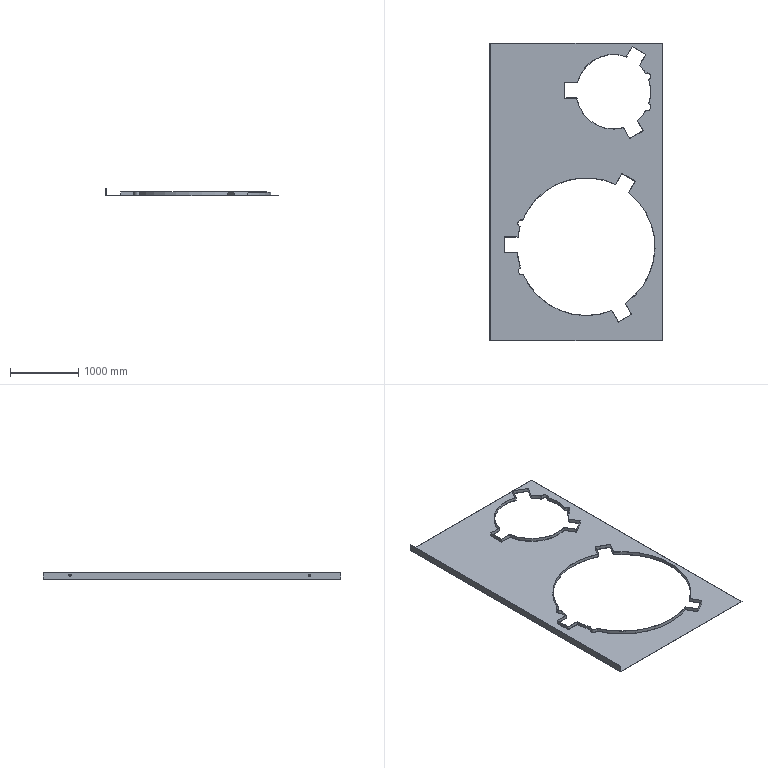Part | STEP file | PN_0023 third-floor right platform deck checkered steel plate_Default<As Machined> | 11 solids | 194 faces | box 2515 x 4350 x 103 mm | volume 22833161 mm3 | plane 144 | cylinder 38 | torus 12 | commonest cylinder face diameters 100 x8 1086 x7 2010 x7 1092 x5 2016 x5 106 x4